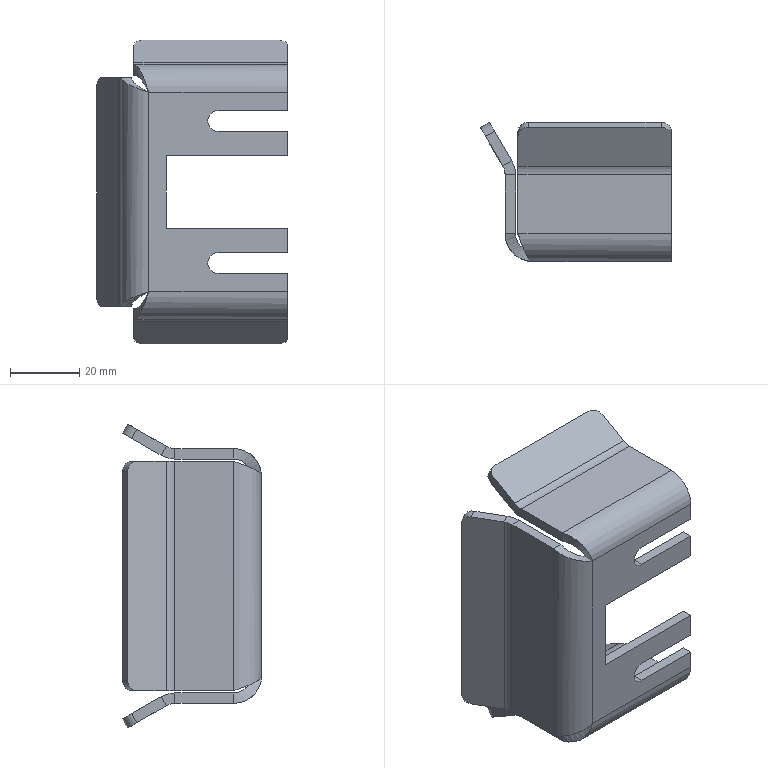Part | NX | features BREP 1 | 1 solid | 72 faces | box 55.098 x 40.134 x 87.696 mm | volume 23763 mm3 | plane 48 | cylinder 20 | spline 4 | commonest cylinder face diameters 6 x8 10 x6 16 x6